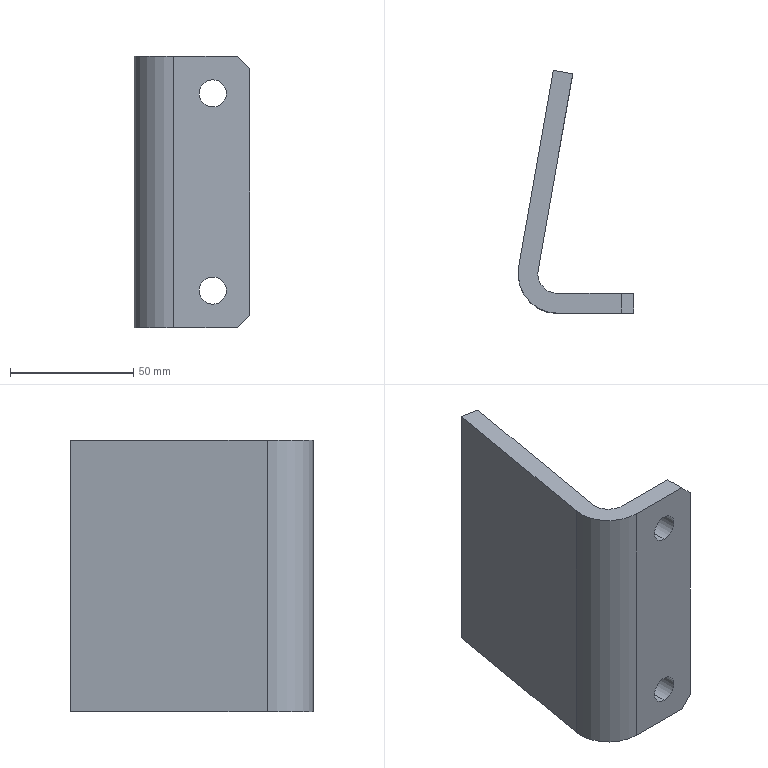Part | SolidWorks | features Fillet 2, Chamfer 1, Extrusion 1, HoleWzd 1, ICE 1 | 1 solid | 16 faces | box 46.932 x 98.481 x 110 mm | volume 115150 mm3 | plane 10 | cylinder 6 | commonest cylinder face diameters 11 x4 16 x1 32 x1
STEP:
#1=CARTESIAN_POINT('',(35.,0.,9.5));
#2=VERTEX_POINT('',#1);
#3=CARTESIAN_POINT('',(35.,0.,20.5));
#4=VERTEX_POINT('',#3);
#5=CARTESIAN_POINT('',(35.,0.,15.));
#6=DIRECTION('',(0.,1.,0.));
#7=DIRECTION('',(0.,0.,1.));
#8=AXIS2_PLACEMENT_3D('',#5,#6,#7);
#9=CIRCLE('',#8,5.5);
#10=EDGE_CURVE('',#2,#4,#9,.T.);
#11=ORIENTED_EDGE('',*,*,#10,.F.);
#12=CARTESIAN_POINT('',(35.,8.,9.5));
#13=VERTEX_POINT('',#12);
#14=CARTESIAN_POINT('',(35.,8.,9.5));
#15=DIRECTION('',(0.,1.,0.));
#16=VECTOR('',#15,1000.);
#17=LINE('',#14,#16);
#18=EDGE_CURVE('',#2,#13,#17,.T.);
#19=ORIENTED_EDGE('',*,*,#18,.T.);
#20=CARTESIAN_POINT('',(35.,8.,20.5));
#21=VERTEX_POINT('',#20);
#22=CARTESIAN_POINT('',(35.,8.,15.));
#23=DIRECTION('',(0.,1.,0.));
#24=DIRECTION('',(0.,0.,1.));
#25=AXIS2_PLACEMENT_3D('',#22,#23,#24);
#26=CIRCLE('',#25,5.5);
#27=EDGE_CURVE('',#13,#21,#26,.T.);
#28=ORIENTED_EDGE('',*,*,#27,.T.);
#29=CARTESIAN_POINT('',(35.,8.,20.5));
#30=DIRECTION('',(0.,1.,0.));
#31=VECTOR('',#30,1000.);
#32=LINE('',#29,#31);
#33=EDGE_CURVE('',#4,#21,#32,.T.);
#34=ORIENTED_EDGE('',*,*,#33,.F.);
#35=EDGE_LOOP('',(#11,#19,#28,#34));
#36=FACE_OUTER_BOUND('',#35,.T.);
#37=CARTESIAN_POINT('',(35.,8.,15.));
#38=DIRECTION('',(0.,1.,0.));
#39=DIRECTION('',(0.,0.,1.));
#40=AXIS2_PLACEMENT_3D('',#37,#38,#39);
#41=CYLINDRICAL_SURFACE('',#40,5.5);
#42=ADVANCED_FACE('',(#36),#41,.F.);
#43=CARTESIAN_POINT('',(35.,0.,89.5));
#44=VERTEX_POINT('',#43);
#45=CARTESIAN_POINT('',(35.,0.,100.5));
#46=VERTEX_POINT('',#45);
#47=CARTESIAN_POINT('',(35.,0.,95.));
#48=DIRECTION('',(0.,1.,0.));
#49=DIRECTION('',(0.,0.,1.));
#50=AXIS2_PLACEMENT_3D('',#47,#48,#49);
#51=CIRCLE('',#50,5.5);
#52=EDGE_CURVE('',#44,#46,#51,.T.);
#53=ORIENTED_EDGE('',*,*,#52,.F.);
#54=CARTESIAN_POINT('',(35.,8.,89.5));
#55=VERTEX_POINT('',#54);
#56=CARTESIAN_POINT('',(35.,8.,89.5));
#57=DIRECTION('',(0.,1.,0.));
#58=VECTOR('',#57,1000.);
#59=LINE('',#56,#58);
#60=EDGE_CURVE('',#44,#55,#59,.T.);
#61=ORIENTED_EDGE('',*,*,#60,.T.);
#62=CARTESIAN_POINT('',(35.,8.,100.5));
#63=VERTEX_POINT('',#62);
#64=CARTESIAN_POINT('',(35.,8.,95.));
#65=DIRECTION('',(0.,1.,0.));
#66=DIRECTION('',(0.,0.,1.));
#67=AXIS2_PLACEMENT_3D('',#64,#65,#66);
#68=CIRCLE('',#67,5.5);
#69=EDGE_CURVE('',#55,#63,#68,.T.);
#70=ORIENTED_EDGE('',*,*,#69,.T.);
#71=CARTESIAN_POINT('',(35.,8.,100.5));
#72=DIRECTION('',(0.,1.,0.));
#73=VECTOR('',#72,1000.);
#74=LINE('',#71,#73);
#75=EDGE_CURVE('',#46,#63,#74,.T.);
#76=ORIENTED_EDGE('',*,*,#75,.F.);
#77=EDGE_LOOP('',(#53,#61,#70,#76));
#78=FACE_OUTER_BOUND('',#77,.T.);
#79=CARTESIAN_POINT('',(35.,8.,95.));
#80=DIRECTION('',(0.,1.,0.));
#81=DIRECTION('',(0.,0.,1.));
#82=AXIS2_PLACEMENT_3D('',#79,#80,#81);
#83=CYLINDRICAL_SURFACE('',#82,5.5);
#84=ADVANCED_FACE('',(#78),#83,.F.);
#85=CARTESIAN_POINT('',(35.,0.,15.));
#86=DIRECTION('',(0.,1.,0.));
#87=DIRECTION('',(0.,0.,1.));
#88=AXIS2_PLACEMENT_3D('',#85,#86,#87);
#89=CIRCLE('',#88,5.5);
#90=EDGE_CURVE('',#4,#2,#89,.T.);
#91=ORIENTED_EDGE('',*,*,#90,.T.);
#92=ORIENTED_EDGE('',*,*,#10,.T.);
#93=EDGE_LOOP('',(#91,#92));
#94=FACE_BOUND('',#93,.T.);
#95=CARTESIAN_POINT('',(35.,0.,95.));
#96=DIRECTION('',(0.,1.,0.));
#97=DIRECTION('',(0.,0.,1.));
#98=AXIS2_PLACEMENT_3D('',#95,#96,#97);
#99=CIRCLE('',#98,5.5);
#100=EDGE_CURVE('',#46,#44,#99,.T.);
#101=ORIENTED_EDGE('',*,*,#100,.T.);
#102=ORIENTED_EDGE('',*,*,#52,.T.);
#103=EDGE_LOOP('',(#101,#102));
#104=FACE_BOUND('',#103,.T.);
#105=CARTESIAN_POINT('',(19.068,0.,110.));
#106=VERTEX_POINT('',#105);
#107=CARTESIAN_POINT('',(45.,0.,110.));
#108=VERTEX_POINT('',#107);
#109=CARTESIAN_POINT('',(0.,0.,110.));
#110=DIRECTION('',(1.,0.,0.));
#111=VECTOR('',#110,1000.);
#112=LINE('',#109,#111);
#113=EDGE_CURVE('',#106,#108,#112,.T.);
#114=ORIENTED_EDGE('',*,*,#113,.F.);
#115=CARTESIAN_POINT('',(19.068,0.,0.));
#116=VERTEX_POINT('',#115);
#117=CARTESIAN_POINT('',(19.068,0.,0.));
#118=DIRECTION('',(0.,0.,-1.));
#119=VECTOR('',#118,1000.);
#120=LINE('',#117,#119);
#121=EDGE_CURVE('',#106,#116,#120,.T.);
#122=ORIENTED_EDGE('',*,*,#121,.T.);
#123=CARTESIAN_POINT('',(45.,0.,0.));
#124=VERTEX_POINT('',#123);
#125=CARTESIAN_POINT('',(0.,0.,0.));
#126=DIRECTION('',(1.,0.,0.));
#127=VECTOR('',#126,1000.);
#128=LINE('',#125,#127);
#129=EDGE_CURVE('',#116,#124,#128,.T.);
#130=ORIENTED_EDGE('',*,*,#129,.T.);
#131=CARTESIAN_POINT('',(50.,0.,5.));
#132=VERTEX_POINT('',#131);
#133=CARTESIAN_POINT('',(22.5,0.,-22.5));
#134=DIRECTION('',(0.7071,0.,0.7071));
#135=VECTOR('',#134,1000.);
#136=LINE('',#133,#135);
#137=EDGE_CURVE('',#124,#132,#136,.T.);
#138=ORIENTED_EDGE('',*,*,#137,.T.);
#139=CARTESIAN_POINT('',(50.,0.,105.));
#140=VERTEX_POINT('',#139);
#141=CARTESIAN_POINT('',(50.,0.,0.));
#142=DIRECTION('',(0.,0.,1.));
#143=VECTOR('',#142,1000.);
#144=LINE('',#141,#143);
#145=EDGE_CURVE('',#132,#140,#144,.T.);
#146=ORIENTED_EDGE('',*,*,#145,.T.);
#147=CARTESIAN_POINT('',(77.5,0.,77.5));
#148=DIRECTION('',(-0.7071,0.,0.7071));
#149=VECTOR('',#148,1000.);
#150=LINE('',#147,#149);
#151=EDGE_CURVE('',#140,#108,#150,.T.);
#152=ORIENTED_EDGE('',*,*,#151,.T.);
#153=EDGE_LOOP('',(#114,#122,#130,#138,#146,#152));
#154=FACE_OUTER_BOUND('',#153,.T.);
#155=CARTESIAN_POINT('',(0.,0.,0.));
#156=DIRECTION('',(0.,-1.,0.));
#157=DIRECTION('',(1.,0.,0.));
#158=AXIS2_PLACEMENT_3D('',#155,#156,#157);
#159=PLANE('',#158);
#160=ADVANCED_FACE('',(#94,#104,#154),#159,.T.);
#161=CARTESIAN_POINT('',(17.365,98.481,0.));
#162=VERTEX_POINT('',#161);
#163=CARTESIAN_POINT('',(3.311,18.778,0.));
#164=VERTEX_POINT('',#163);
#165=CARTESIAN_POINT('',(17.365,98.481,0.));
#166=DIRECTION('',(-0.1736,-0.9848,0.));
#167=VECTOR('',#166,1000.);
#168=LINE('',#165,#167);
#169=EDGE_CURVE('',#162,#164,#168,.T.);
#170=ORIENTED_EDGE('',*,*,#169,.T.);
#171=CARTESIAN_POINT('',(3.311,18.778,110.));
#172=VERTEX_POINT('',#171);
#173=CARTESIAN_POINT('',(3.311,18.778,0.));
#174=DIRECTION('',(0.,0.,1.));
#175=VECTOR('',#174,1000.);
#176=LINE('',#173,#175);
#177=EDGE_CURVE('',#164,#172,#176,.T.);
#178=ORIENTED_EDGE('',*,*,#177,.T.);
#179=CARTESIAN_POINT('',(17.365,98.481,110.));
#180=VERTEX_POINT('',#179);
#181=CARTESIAN_POINT('',(17.365,98.481,110.));
#182=DIRECTION('',(-0.1736,-0.9848,0.));
#183=VECTOR('',#182,1000.);
#184=LINE('',#181,#183);
#185=EDGE_CURVE('',#180,#172,#184,.T.);
#186=ORIENTED_EDGE('',*,*,#185,.F.);
#187=CARTESIAN_POINT('',(17.365,98.481,0.));
#188=DIRECTION('',(0.,0.,1.));
#189=VECTOR('',#188,1000.);
#190=LINE('',#187,#189);
#191=EDGE_CURVE('',#162,#180,#190,.T.);
#192=ORIENTED_EDGE('',*,*,#191,.F.);
#193=EDGE_LOOP('',(#170,#178,#186,#192));
#194=FACE_OUTER_BOUND('',#193,.T.);
#195=CARTESIAN_POINT('',(17.365,98.481,0.));
#196=DIRECTION('',(-0.9848,0.1736,0.));
#197=DIRECTION('',(-0.1736,-0.9848,0.));
#198=AXIS2_PLACEMENT_3D('',#195,#196,#197);
#199=PLANE('',#198);
#200=ADVANCED_FACE('',(#194),#199,.T.);
#201=CARTESIAN_POINT('',(25.243,97.092,110.));
#202=VERTEX_POINT('',#201);
#203=CARTESIAN_POINT('',(25.243,97.092,0.));
#204=VERTEX_POINT('',#203);
#205=CARTESIAN_POINT('',(25.243,97.092,110.));
#206=DIRECTION('',(0.,0.,-1.));
#207=VECTOR('',#206,1000.);
#208=LINE('',#205,#207);
#209=EDGE_CURVE('',#202,#204,#208,.T.);
#210=ORIENTED_EDGE('',*,*,#209,.T.);
#211=CARTESIAN_POINT('',(50.,92.726,0.));
#212=DIRECTION('',(-0.9848,0.1736,0.));
#213=VECTOR('',#212,1000.);
#214=LINE('',#211,#213);
#215=EDGE_CURVE('',#204,#162,#214,.T.);
#216=ORIENTED_EDGE('',*,*,#215,.T.);
#217=ORIENTED_EDGE('',*,*,#191,.T.);
#218=CARTESIAN_POINT('',(50.,92.726,110.));
#219=DIRECTION('',(-0.9848,0.1736,0.));
#220=VECTOR('',#219,1000.);
#221=LINE('',#218,#220);
#222=EDGE_CURVE('',#202,#180,#221,.T.);
#223=ORIENTED_EDGE('',*,*,#222,.F.);
#224=EDGE_LOOP('',(#210,#216,#217,#223));
#225=FACE_OUTER_BOUND('',#224,.T.);
#226=CARTESIAN_POINT('',(50.,92.726,0.));
#227=DIRECTION('',(0.1736,0.9848,0.));
#228=DIRECTION('',(-0.9848,0.1736,0.));
#229=AXIS2_PLACEMENT_3D('',#226,#227,#228);
#230=PLANE('',#229);
#231=ADVANCED_FACE('',(#225),#230,.T.);
#232=ORIENTED_EDGE('',*,*,#145,.F.);
#233=CARTESIAN_POINT('',(50.,8.,5.));
#234=VERTEX_POINT('',#233);
#235=CARTESIAN_POINT('',(50.,8.,5.));
#236=DIRECTION('',(0.,1.,0.));
#237=VECTOR('',#236,1000.);
#238=LINE('',#235,#237);
#239=EDGE_CURVE('',#132,#234,#238,.T.);
#240=ORIENTED_EDGE('',*,*,#239,.T.);
#241=CARTESIAN_POINT('',(50.,8.,105.));
#242=VERTEX_POINT('',#241);
#243=CARTESIAN_POINT('',(50.,8.,110.));
#244=DIRECTION('',(0.,0.,-1.));
#245=VECTOR('',#244,1000.);
#246=LINE('',#243,#245);
#247=EDGE_CURVE('',#242,#234,#246,.T.);
#248=ORIENTED_EDGE('',*,*,#247,.F.);
#249=CARTESIAN_POINT('',(50.,0.,105.));
#250=DIRECTION('',(0.,-1.,0.));
#251=VECTOR('',#250,1000.);
#252=LINE('',#249,#251);
#253=EDGE_CURVE('',#242,#140,#252,.T.);
#254=ORIENTED_EDGE('',*,*,#253,.T.);
#255=EDGE_LOOP('',(#232,#240,#248,#254));
#256=FACE_OUTER_BOUND('',#255,.T.);
#257=CARTESIAN_POINT('',(50.,0.,0.));
#258=DIRECTION('',(1.,0.,0.));
#259=DIRECTION('',(0.,1.,0.));
#260=AXIS2_PLACEMENT_3D('',#257,#258,#259);
#261=PLANE('',#260);
#262=ADVANCED_FACE('',(#256),#261,.T.);
#263=ORIENTED_EDGE('',*,*,#129,.F.);
#264=CARTESIAN_POINT('',(19.068,16.,0.));
#265=DIRECTION('',(0.,0.,-1.));
#266=DIRECTION('',(1.,0.,0.));
#267=AXIS2_PLACEMENT_3D('',#264,#265,#266);
#268=CIRCLE('',#267,16.);
#269=EDGE_CURVE('',#116,#164,#268,.T.);
#270=ORIENTED_EDGE('',*,*,#269,.T.);
#271=ORIENTED_EDGE('',*,*,#169,.F.);
#272=ORIENTED_EDGE('',*,*,#215,.F.);
#273=CARTESIAN_POINT('',(11.19,17.389,0.));
#274=VERTEX_POINT('',#273);
#275=CARTESIAN_POINT('',(9.534,8.,0.));
#276=DIRECTION('',(0.1736,0.9848,0.));
#277=VECTOR('',#276,1000.);
#278=LINE('',#275,#277);
#279=EDGE_CURVE('',#274,#204,#278,.T.);
#280=ORIENTED_EDGE('',*,*,#279,.F.);
#281=CARTESIAN_POINT('',(19.068,8.,0.));
#282=VERTEX_POINT('',#281);
#283=CARTESIAN_POINT('',(19.068,16.,0.));
#284=DIRECTION('',(0.,0.,1.));
#285=DIRECTION('',(1.,0.,0.));
#286=AXIS2_PLACEMENT_3D('',#283,#284,#285);
#287=CIRCLE('',#286,8.);
#288=EDGE_CURVE('',#274,#282,#287,.T.);
#289=ORIENTED_EDGE('',*,*,#288,.T.);
#290=CARTESIAN_POINT('',(45.,8.,0.));
#291=VERTEX_POINT('',#290);
#292=CARTESIAN_POINT('',(50.,8.,0.));
#293=DIRECTION('',(-1.,0.,0.));
#294=VECTOR('',#293,1000.);
#295=LINE('',#292,#294);
#296=EDGE_CURVE('',#291,#282,#295,.T.);
#297=ORIENTED_EDGE('',*,*,#296,.F.);
#298=CARTESIAN_POINT('',(45.,0.,0.));
#299=DIRECTION('',(0.,-1.,0.));
#300=VECTOR('',#299,1000.);
#301=LINE('',#298,#300);
#302=EDGE_CURVE('',#291,#124,#301,.T.);
#303=ORIENTED_EDGE('',*,*,#302,.T.);
#304=EDGE_LOOP('',(#263,#270,#271,#272,#280,#289,#297,#303));
#305=FACE_OUTER_BOUND('',#304,.T.);
#306=CARTESIAN_POINT('',(0.,0.,0.));
#307=DIRECTION('',(0.,0.,1.));
#308=DIRECTION('',(1.,0.,0.));
#309=AXIS2_PLACEMENT_3D('',#306,#307,#308);
#310=PLANE('',#309);
#311=ADVANCED_FACE('',(#305),#310,.F.);
#312=ORIENTED_EDGE('',*,*,#185,.T.);
#313=CARTESIAN_POINT('',(19.068,16.,110.));
#314=DIRECTION('',(0.,0.,1.));
#315=DIRECTION('',(1.,0.,0.));
#316=AXIS2_PLACEMENT_3D('',#313,#314,#315);
#317=CIRCLE('',#316,16.);
#318=EDGE_CURVE('',#172,#106,#317,.T.);
#319=ORIENTED_EDGE('',*,*,#318,.T.);
#320=ORIENTED_EDGE('',*,*,#113,.T.);
#321=CARTESIAN_POINT('',(45.,8.,110.));
#322=VERTEX_POINT('',#321);
#323=CARTESIAN_POINT('',(45.,0.,110.));
#324=DIRECTION('',(0.,1.,0.));
#325=VECTOR('',#324,1000.);
#326=LINE('',#323,#325);
#327=EDGE_CURVE('',#108,#322,#326,.T.);
#328=ORIENTED_EDGE('',*,*,#327,.T.);
#329=CARTESIAN_POINT('',(19.068,8.,110.));
#330=VERTEX_POINT('',#329);
#331=CARTESIAN_POINT('',(50.,8.,110.));
#332=DIRECTION('',(-1.,0.,0.));
#333=VECTOR('',#332,1000.);
#334=LINE('',#331,#333);
#335=EDGE_CURVE('',#322,#330,#334,.T.);
#336=ORIENTED_EDGE('',*,*,#335,.T.);
#337=CARTESIAN_POINT('',(11.19,17.389,110.));
#338=VERTEX_POINT('',#337);
#339=CARTESIAN_POINT('',(19.068,16.,110.));
#340=DIRECTION('',(0.,0.,-1.));
#341=DIRECTION('',(1.,0.,0.));
#342=AXIS2_PLACEMENT_3D('',#339,#340,#341);
#343=CIRCLE('',#342,8.);
#344=EDGE_CURVE('',#330,#338,#343,.T.);
#345=ORIENTED_EDGE('',*,*,#344,.T.);
#346=CARTESIAN_POINT('',(9.534,8.,110.));
#347=DIRECTION('',(0.1736,0.9848,0.));
#348=VECTOR('',#347,1000.);
#349=LINE('',#346,#348);
#350=EDGE_CURVE('',#338,#202,#349,.T.);
#351=ORIENTED_EDGE('',*,*,#350,.T.);
#352=ORIENTED_EDGE('',*,*,#222,.T.);
#353=EDGE_LOOP('',(#312,#319,#320,#328,#336,#345,#351,#352));
#354=FACE_OUTER_BOUND('',#353,.T.);
#355=CARTESIAN_POINT('',(0.,0.,110.));
#356=DIRECTION('',(0.,0.,1.));
#357=DIRECTION('',(1.,0.,0.));
#358=AXIS2_PLACEMENT_3D('',#355,#356,#357);
#359=PLANE('',#358);
#360=ADVANCED_FACE('',(#354),#359,.T.);
#361=CARTESIAN_POINT('',(35.,8.,15.));
#362=DIRECTION('',(0.,1.,0.));
#363=DIRECTION('',(0.,0.,1.));
#364=AXIS2_PLACEMENT_3D('',#361,#362,#363);
#365=CIRCLE('',#364,5.5);
#366=EDGE_CURVE('',#21,#13,#365,.T.);
#367=ORIENTED_EDGE('',*,*,#366,.F.);
#368=ORIENTED_EDGE('',*,*,#27,.F.);
#369=EDGE_LOOP('',(#367,#368));
#370=FACE_BOUND('',#369,.T.);
#371=CARTESIAN_POINT('',(35.,8.,95.));
#372=DIRECTION('',(0.,1.,0.));
#373=DIRECTION('',(0.,0.,1.));
#374=AXIS2_PLACEMENT_3D('',#371,#372,#373);
#375=CIRCLE('',#374,5.5);
#376=EDGE_CURVE('',#63,#55,#375,.T.);
#377=ORIENTED_EDGE('',*,*,#376,.F.);
#378=ORIENTED_EDGE('',*,*,#69,.F.);
#379=EDGE_LOOP('',(#377,#378));
#380=FACE_BOUND('',#379,.T.);
#381=ORIENTED_EDGE('',*,*,#296,.T.);
#382=CARTESIAN_POINT('',(19.068,8.,110.));
#383=DIRECTION('',(0.,0.,1.));
#384=VECTOR('',#383,1000.);
#385=LINE('',#382,#384);
#386=EDGE_CURVE('',#282,#330,#385,.T.);
#387=ORIENTED_EDGE('',*,*,#386,.T.);
#388=ORIENTED_EDGE('',*,*,#335,.F.);
#389=CARTESIAN_POINT('',(45.,8.,110.));
#390=DIRECTION('',(0.7071,0.,-0.7071));
#391=VECTOR('',#390,1000.);
#392=LINE('',#389,#391);
#393=EDGE_CURVE('',#322,#242,#392,.T.);
#394=ORIENTED_EDGE('',*,*,#393,.T.);
#395=ORIENTED_EDGE('',*,*,#247,.T.);
#396=CARTESIAN_POINT('',(50.,8.,5.));
#397=DIRECTION('',(-0.7071,0.,-0.7071));
#398=VECTOR('',#397,1000.);
#399=LINE('',#396,#398);
#400=EDGE_CURVE('',#234,#291,#399,.T.);
#401=ORIENTED_EDGE('',*,*,#400,.T.);
#402=EDGE_LOOP('',(#381,#387,#388,#394,#395,#401));
#403=FACE_OUTER_BOUND('',#402,.T.);
#404=CARTESIAN_POINT('',(50.,8.,110.));
#405=DIRECTION('',(0.,-1.,0.));
#406=DIRECTION('',(0.,0.,-1.));
#407=AXIS2_PLACEMENT_3D('',#404,#405,#406);
#408=PLANE('',#407);
#409=ADVANCED_FACE('',(#370,#380,#403),#408,.F.);
#410=ORIENTED_EDGE('',*,*,#350,.F.);
#411=CARTESIAN_POINT('',(11.19,17.389,0.));
#412=DIRECTION('',(0.,0.,-1.));
#413=VECTOR('',#412,1000.);
#414=LINE('',#411,#413);
#415=EDGE_CURVE('',#338,#274,#414,.T.);
#416=ORIENTED_EDGE('',*,*,#415,.T.);
#417=ORIENTED_EDGE('',*,*,#279,.T.);
#418=ORIENTED_EDGE('',*,*,#209,.F.);
#419=EDGE_LOOP('',(#410,#416,#417,#418));
#420=FACE_OUTER_BOUND('',#419,.T.);
#421=CARTESIAN_POINT('',(9.534,8.,110.));
#422=DIRECTION('',(-0.9848,0.1736,0.));
#423=DIRECTION('',(-0.1736,-0.9848,0.));
#424=AXIS2_PLACEMENT_3D('',#421,#422,#423);
#425=PLANE('',#424);
#426=ADVANCED_FACE('',(#420),#425,.F.);
#427=ORIENTED_EDGE('',*,*,#60,.F.);
#428=ORIENTED_EDGE('',*,*,#100,.F.);
#429=ORIENTED_EDGE('',*,*,#75,.T.);
#430=ORIENTED_EDGE('',*,*,#376,.T.);
#431=EDGE_LOOP('',(#427,#428,#429,#430));
#432=FACE_OUTER_BOUND('',#431,.T.);
#433=CARTESIAN_POINT('',(35.,8.,95.));
#434=DIRECTION('',(0.,1.,0.));
#435=DIRECTION('',(0.,0.,1.));
#436=AXIS2_PLACEMENT_3D('',#433,#434,#435);
#437=CYLINDRICAL_SURFACE('',#436,5.5);
#438=ADVANCED_FACE('',(#432),#437,.F.);
#439=ORIENTED_EDGE('',*,*,#18,.F.);
#440=ORIENTED_EDGE('',*,*,#90,.F.);
#441=ORIENTED_EDGE('',*,*,#33,.T.);
#442=ORIENTED_EDGE('',*,*,#366,.T.);
#443=EDGE_LOOP('',(#439,#440,#441,#442));
#444=FACE_OUTER_BOUND('',#443,.T.);
#445=CARTESIAN_POINT('',(35.,8.,15.));
#446=DIRECTION('',(0.,1.,0.));
#447=DIRECTION('',(0.,0.,1.));
#448=AXIS2_PLACEMENT_3D('',#445,#446,#447);
#449=CYLINDRICAL_SURFACE('',#448,5.5);
#450=ADVANCED_FACE('',(#444),#449,.F.);
#451=ORIENTED_EDGE('',*,*,#137,.F.);
#452=ORIENTED_EDGE('',*,*,#302,.F.);
#453=ORIENTED_EDGE('',*,*,#400,.F.);
#454=ORIENTED_EDGE('',*,*,#239,.F.);
#455=EDGE_LOOP('',(#451,#452,#453,#454));
#456=FACE_OUTER_BOUND('',#455,.T.);
#457=CARTESIAN_POINT('',(50.,0.,5.));
#458=DIRECTION('',(0.7071,0.,-0.7071));
#459=DIRECTION('',(0.,-1.,0.));
#460=AXIS2_PLACEMENT_3D('',#457,#458,#459);
#461=PLANE('',#460);
#462=ADVANCED_FACE('',(#456),#461,.T.);
#463=ORIENTED_EDGE('',*,*,#151,.F.);
#464=ORIENTED_EDGE('',*,*,#253,.F.);
#465=ORIENTED_EDGE('',*,*,#393,.F.);
#466=ORIENTED_EDGE('',*,*,#327,.F.);
#467=EDGE_LOOP('',(#463,#464,#465,#466));
#468=FACE_OUTER_BOUND('',#467,.T.);
#469=CARTESIAN_POINT('',(45.,0.,110.));
#470=DIRECTION('',(-0.7071,0.,-0.7071));
#471=DIRECTION('',(0.,1.,0.));
#472=AXIS2_PLACEMENT_3D('',#469,#470,#471);
#473=PLANE('',#472);
#474=ADVANCED_FACE('',(#468),#473,.F.);
#475=ORIENTED_EDGE('',*,*,#344,.F.);
#476=ORIENTED_EDGE('',*,*,#386,.F.);
#477=ORIENTED_EDGE('',*,*,#288,.F.);
#478=ORIENTED_EDGE('',*,*,#415,.F.);
#479=EDGE_LOOP('',(#475,#476,#477,#478));
#480=FACE_OUTER_BOUND('',#479,.T.);
#481=CARTESIAN_POINT('',(19.068,16.,110.));
#482=DIRECTION('',(0.,0.,1.));
#483=DIRECTION('',(1.,0.,0.));
#484=AXIS2_PLACEMENT_3D('',#481,#482,#483);
#485=CYLINDRICAL_SURFACE('',#484,8.);
#486=ADVANCED_FACE('',(#480),#485,.F.);
#487=ORIENTED_EDGE('',*,*,#269,.F.);
#488=ORIENTED_EDGE('',*,*,#121,.F.);
#489=ORIENTED_EDGE('',*,*,#318,.F.);
#490=ORIENTED_EDGE('',*,*,#177,.F.);
#491=EDGE_LOOP('',(#487,#488,#489,#490));
#492=FACE_OUTER_BOUND('',#491,.T.);
#493=CARTESIAN_POINT('',(19.068,16.,0.));
#494=DIRECTION('',(0.,0.,1.));
#495=DIRECTION('',(1.,0.,0.));
#496=AXIS2_PLACEMENT_3D('',#493,#494,#495);
#497=CYLINDRICAL_SURFACE('',#496,16.);
#498=ADVANCED_FACE('',(#492),#497,.T.);
#499=CLOSED_SHELL('',(#42,#84,#160,#200,#231,#262,#311,#360,#409,#426,#438,#450,#462,#474,#486,#498));
#500=MANIFOLD_SOLID_BREP('',#499);
#501=CARTESIAN_POINT('',(0.,0.,0.));
#502=DIRECTION('',(0.,0.,1.));
#503=DIRECTION('',(1.,0.,0.));
#504=AXIS2_PLACEMENT_3D('',#501,#502,#503);
#505=(LENGTH_UNIT()NAMED_UNIT(*)SI_UNIT(.MILLI.,.METRE.));
#506=UNCERTAINTY_MEASURE_WITH_UNIT(LENGTH_MEASURE(0.00001),#505,'','');
#507=(NAMED_UNIT(*)PLANE_ANGLE_UNIT()SI_UNIT($,.RADIAN.));
#508=(NAMED_UNIT(*)SI_UNIT($,.STERADIAN.)SOLID_ANGLE_UNIT());
#509=(GEOMETRIC_REPRESENTATION_CONTEXT(3)GLOBAL_UNCERTAINTY_ASSIGNED_CONTEXT((#506))GLOBAL_UNIT_ASSIGNED_CONTEXT((#505,#507,#508))REPRESENTATION_CONTEXT('',''));
#510=ADVANCED_BREP_SHAPE_REPRESENTATION('',(#500,#504),#509);